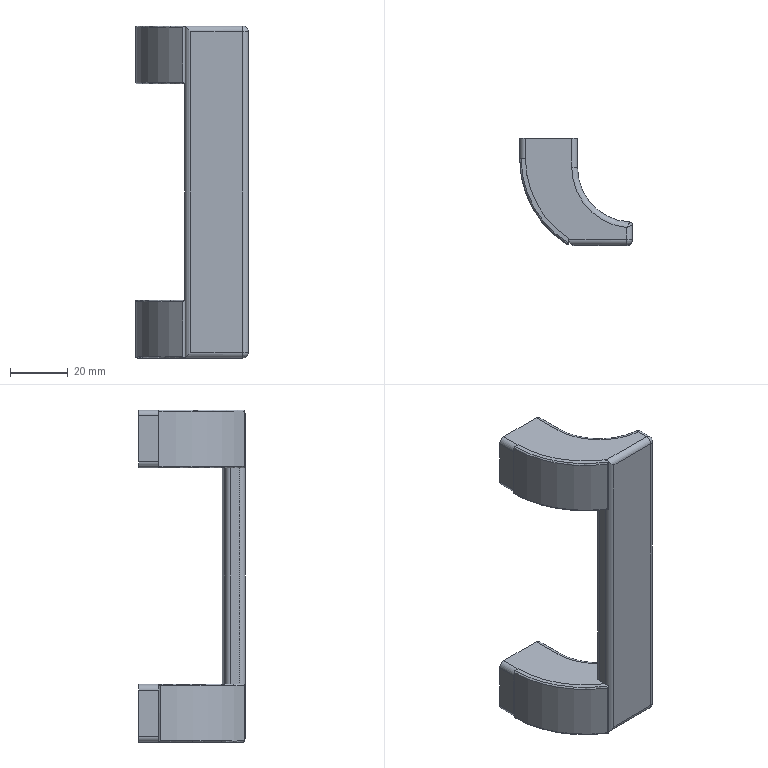Part | STEP file | 3 solids | 94 faces | box 39 x 37 x 115 mm | volume 35258 mm3 | plane 41 | cylinder 39 | torus 8 | spline 4 | sphere 2 | commonest cylinder face diameters 4 x15 1 x4 6.6 x4 11 x4 65.941 x4 2 x3